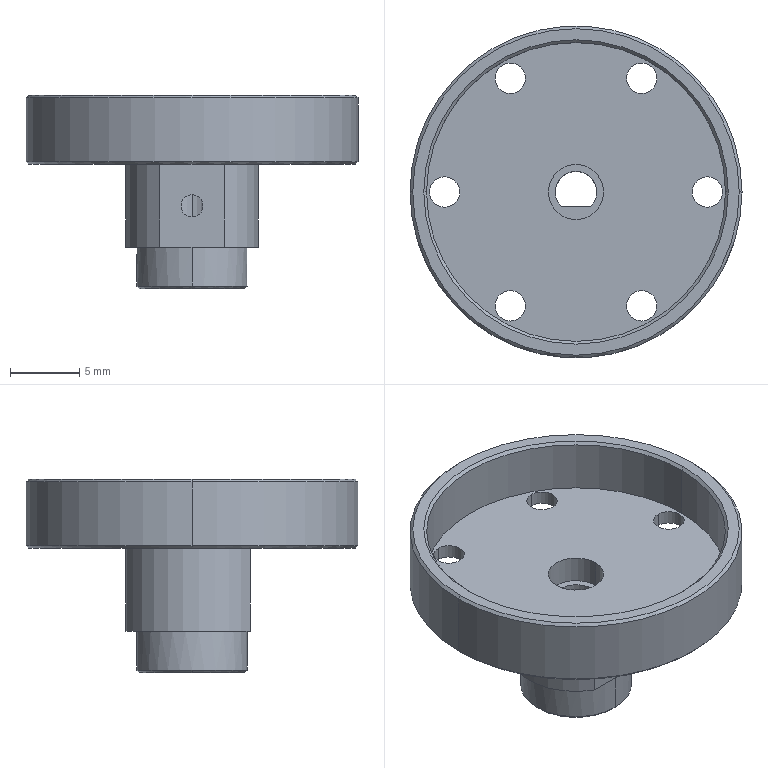NC program | NX | posted with a generic post | part box 24 x 24 x 14 mm
Whole program:
N10 G17 G21 G94 G90
(FLOOR_WALL , TOOL : D80)
N12 T19 M6
N14 G54
N16 G17 G0 G90 X-60. Y0. S6500 M3
N18 G43 Z30. H19
N20 Z3.
N22 G94 G1 Z0. F1500.
N24 X-57.
N26 X57.
N28 X60.
N30 Z3.
N32 G0 Z30.
N34 M5
(ADAPTIVE_MILLING , TOOL : D10)
N36 T15 M6
N38 G54
N40 G17 G0 G90 X-24.709 Y0.063 S9500 M3
N42 G43 Z30. H15
N44 Z-11.
N46 G94 G1 Z-14. F1000.
N48 X-23.929 Y-0.217 F3000.
N50 X-23.14 Y-0.473
N52 G3 X-22.062 Y0.063 R1.017
N54 X-21.301 Y3.126 R8.28
N56 X-21.019 Y12.993 R111.643
N58 G2 X-20.631 Y15.815 R6.542
N60 X-16.684 Y19.458 R7.316
N62 X-10.226 Y20.78 R19.548
N64 X2.021 Y20.985 R218.689
N66 X14.52 Y20.957 R545.112
N68 X18.704 Y18.063 R6.07
N70 X20.563 Y12.41 R13.683
N72 X20.97 Y3.05 R80.124
N74 G1 X20.978 Y1.55
N76 X20.983 Y-0.575
N78 X20.987 Y-3.825
N80 X20.988 Y-11.575
N82 Y-14.075
N84 X20.984 Y-14.2
N86 X20.977 Y-14.325
N88 X20.965 Y-14.45
N90 G2 X18.123 Y-18.666 R6.024
N92 X12.356 Y-20.57 R13.682
N94 X3.746 Y-20.965 R75.213
N96 G1 X2.621 Y-20.973
N98 X0.996 Y-20.98
N100 X-1.129 Y-20.984
N102 X-4.879 Y-20.987
N104 X-14.004 Y-20.988
N106 X-14.129 Y-20.986
N108 G2 X-18.331 Y-18.583 R5.703
N110 X-20.484 Y-12.917 R12.28
N112 X-20.964 Y-3.813 R67.206
N114 X-20.499 Y1.413 R49.975
N116 G3 X-20.03 Y11.524 R121.229
N118 G2 X-16.346 Y17.329 R7.752
N120 X-10.001 Y19.468 R15.489
N122 X-0.145 Y19.951 R80.815
N124 X11.604 Y19.947 R639.978
N126 X17.379 Y16.22 R7.712
N128 X19.482 Y9.861 R15.761
N130 X19.954 Y-0.247 R84.683
N132 X19.946 Y-11.621 R553.653
N134 X16.206 Y-17.388 R7.727
N136 X9.72 Y-19.498 R15.834
N138 X0.362 Y-19.949 R79.462
N140 X-11.637 Y-19.945 R478.691
N142 X-17.461 Y-16.084 R7.744
N144 X-19.515 Y-9.578 R16.213
N146 X-19.566 Y0.15 R42.335
N148 G3 X-19.067 Y9.385 R295.109
N150 G2 X-14.18 Y16.505 R9.108
N152 X-7.382 Y18.489 R18.641
N154 X3.103 Y18.942 R98.39
N156 X9.601 Y18.901 R98.045
N158 X16.439 Y14.21 R8.937
N160 X18.49 Y7.307 R18.265
N162 X18.94 Y-2.928 R95.698
N164 X18.906 Y-9.551 R109.181
N166 X14.255 Y-16.415 R8.913
N168 X7.233 Y-18.501 R18.411
N170 X-2.627 Y-18.937 R93.906
N172 X-9.5 Y-18.909 R118.757
N174 X-16.448 Y-14.185 R8.923
N176 X-18.535 Y-6.653 R18.416
N178 X-18.443 Y1.215 R58.227
N180 X-18.079 Y7.828 R136.173
N182 X-12.507 Y15.497 R10.026
N184 X-5.44 Y17.462 R20.584
N186 X7.418 Y17.888 R103.688
N188 X15.323 Y12.702 R9.73
N190 X17.406 Y5.803 R19.282
N192 X17.917 Y-4.303 R87.187
N194 X17.696 Y-8.788 R21.352
N196 X12.475 Y-15.447 R9.836
N198 X5.299 Y-17.472 R20.106
N200 X-7.435 Y-17.885 R103.812
N202 X-15.329 Y-12.682 R9.719
N204 X-17.376 Y-4.891 R18.076
N206 X-17.104 Y6.222 R84.007
N208 X-10.954 Y14.491 R10.754
N210 X-5.591 Y16.165 R19.739
N212 G1 X-4.308 Y16.597
N214 X-4.233 Y16.617
N216 X-1.841 Y17.048
N218 X-1.764 Y17.056
N220 G2 X3.23 Y17.012 R41.186
N222 X8.297 Y16.393 R17.013
N224 X14.624 Y10.53 R10.801
N226 X16.111 Y5.758 R19.717
N228 G1 X16.487 Y4.713
N230 X16.507 Y4.643
N232 G2 X17.149 Y0.012 R19.905
N234 G3 X16.904 Y-5.606 R192.191
N236 G2 X11.08 Y-14.346 R10.491
N238 X5.747 Y-16.114 R18.666
N240 G1 X4.848 Y-16.448
N242 X4.776 Y-16.469
N244 G2 X-0.019 Y-17.149 R19.964
N246 G3 X-5.637 Y-16.902 R229.027
N248 G2 X-14.514 Y-10.707 R10.491
N250 X-15.859 Y-6.426 R17.286
N252 G1 X-16.437 Y-4.886
N254 X-16.458 Y-4.812
N256 G2 X-17.148 Y0.051 R19.974
N258 G1 X-16.965 Y2.493
N260 X-16.954 Y2.57
N262 G2 X-15.648 Y7.316 R27.58
N264 X-13.008 Y11.136 R11.482
N266 X-10.896 Y13.241 R19.934
N268 G1 X-8.914 Y14.648
N270 X-8.848 Y14.688
N272 X-6.683 Y15.791
N274 X-6.611 Y15.821
N276 X-5.545 Y16.181
N278 X-4.233 Y16.617
N280 X-1.764 Y17.056
N282 X0.734 Y17.132
N284 X3.156 Y16.854
N286 X3.233 Y16.84
N288 G2 X8.077 Y15.188 R22.325
N290 X13.269 Y10.861 R19.685
N292 X15.717 Y6.857 R19.804
N294 G1 X16.139 Y5.681
N296 G3 X17.954 Y6.829 R-1.1
N298 G1 X6.864 Y17.977
N300 G3 X5.653 Y16.189 R-1.1
N302 G2 X9.829 Y14.051 R19.797
N304 G1 X10.413 Y13.581
N306 X11.659 Y12.574
N308 G2 X14.631 Y8.943 R20.021
N310 X16.507 Y4.643 R20.021
N312 X17.149 Y0.012 R20.111
N314 G1 X16.979 Y-2.397
N316 X16.968 Y-2.472
N318 G2 X15.096 Y-8.247 R20.663
N320 X13.544 Y-10.451 R12.904
N322 G1 X12.945 Y-11.245
N324 X12.896 Y-11.302
N326 G2 X9.206 Y-14.467 R19.857
N328 G1 X7.131 Y-15.594
N330 X7.062 Y-15.625
N332 X5.656 Y-16.148
N334 G3 X6.833 Y-17.941 R-1.1
N336 G1 X18.26 Y-6.034
N338 G3 X16.437 Y-4.886 R-1.1
N340 G2 X14.368 Y-9.36 R19.883
N342 G1 X13.539 Y-10.457
N344 X12.896 Y-11.302
N346 X11.164 Y-13.016
N348 X9.206 Y-14.467
N350 X7.062 Y-15.625
N352 X4.776 Y-16.469
N354 X2.393 Y-16.98
N356 X-0.019 Y-17.149
N358 X-2.393 Y-16.98
N360 X-2.468 Y-16.969
N362 G2 X-8.322 Y-15.053 R20.327
N364 X-10.38 Y-13.599 R12.851
N366 G1 X-11.164 Y-13.016
N368 X-11.221 Y-12.966
N370 G2 X-14.409 Y-9.296 R19.854
N372 G1 X-15.564 Y-7.198
N374 X-15.596 Y-7.128
N376 X-15.859 Y-6.426
N378 G3 X-17.631 Y-7.624 R-1.1
N380 G1 X-5.974 Y-18.29
N382 G3 X-4.848 Y-16.448 R-1.1
N384 G2 X-9.269 Y-14.426 R19.857
N386 G1 X-10.473 Y-13.53
N388 G3 X-11.229 Y-13.345 R1.027
N390 G1 X-11.962 Y-13.464
N392 X-13.937 Y-13.783 Z-13.9
N394 G2 X-14.973 Y-13.53 R1.086
N396 X-16.017 Y-12.377 R9.067
N398 G1 X-16.944 Y-10.932
N400 X-17.851 Y-9.475
N402 G2 X-19.849 Y-2.989 R15.613
N404 G1 X-20.317 Y2.69
N406 G2 X-19.529 Y3.751 R1.005
N408 G1 X-19.251 Y3.81
N410 X-17.295 Y4.226 Z-14.
N412 G3 X-16.42 Y4.94 R1.044
N414 G1 X-16.398 Y5.015
N416 X-15.524 Y7.282
N418 X-15.491 Y7.353
N420 X-14.296 Y9.469
N422 X-14.253 Y9.533
N424 X-12.949 Y11.211
N426 G3 X-12.926 Y12.419 R1.017
N428 G1 X-13.921 Y13.807
N430 Z-11.
N432 G0 Z30.
(ADAPTIVE_MILLING_COPY , TOOL : D10)
N434 X3.265 Y3.084
N436 Z3.
N438 G3 X3.265 Y3.084 Z2.506 I-3.272 J-3.089 F1000.
N440 X3.265 Y3.084 Z2.013 I-3.272 J-3.089
N442 X3.265 Y3.084 Z1.519 I-3.272 J-3.089
N444 X3.265 Y3.084 Z1.026 I-3.272 J-3.089
N446 X3.265 Y3.084 Z0.532 I-3.272 J-3.089
N448 X3.265 Y3.084 Z0.039 I-3.272 J-3.089
N450 X3.265 Y3.084 Z-0.455 I-3.272 J-3.089
N452 X3.265 Y3.084 Z-0.948 I-3.272 J-3.089
N454 X3.265 Y3.084 Z-1.442 I-3.272 J-3.089
N456 X3.265 Y3.084 Z-1.935 I-3.272 J-3.089
N458 X3.265 Y3.084 Z-2.429 I-3.272 J-3.089
N460 X3.265 Y3.084 Z-2.922 I-3.272 J-3.089
N462 X3.265 Y3.084 Z-3.416 I-3.272 J-3.089
N464 X4.493 Y-0.005 Z-3.85 R-4.5
N466 X3.671 Y-2.611 R-4.501 F3000.
N468 X-0.999 Y4.865 R4.671
N470 X3.576 Y-3.479 R-4.978
N472 X-1.657 Y5.205 R5.195
N474 X3.671 Y-4.091 R-5.477
N476 X5.235 Y-1.957 R5.961
N478 X5.632 Y0.167 R5.3
N480 X0.038 Y5.633 R5.695
N482 X-4.908 Y2.763 R5.788
N484 X-5.483 Y-1.313 R5.926
N486 X5.499 Y-1.168 R5.633
N488 X4.493 Y-0.032 R1.014
N490 G1 X3.116 Y-0.038
N492 Z-0.85
N494 G0 Z30.
N496 M5
(ZLEVEL_PROFILE_COPY_1_COPY_COPY_1 , TOOL : D10JING)
N498 T14 M6
N500 G54
N502 G17 G0 G90 X-18.925 Y-1.689 S9500 M3
N504 G43 Z30. H14
N506 Z-13.
N508 G94 G1 Z-14. F1000.
N510 X-17.5 Y-0.866
N512 G3 X-17. Y0. R1.
N514 G1 Y0.024 F1200.
N516 G2 X0.024 Y17. R17.
N518 X-17. Y0. R-17.
N520 G3 X-17.5 Y0.866 R1.
N522 G1 X-18.925 Y1.689
N524 Z-13.
N526 G0 Z30.
(FLOOR_WALL_1 , TOOL : D10JING)
N528 X0. Y-2.8
N530 Z-1.
N532 G1 Z-4. F1250.
N534 Y0.2
N536 G3 X-0.2 Y0. R0.2
N538 X0. Y0.2 R-0.2
N540 G1 Y5.2
N542 G3 X-5.2 Y0. R5.2
N544 X0. Y5.2 R-5.2
N546 G1 Y2.2
N548 Y5.7
N550 G3 X-5.7 Y0. R5.7
N552 X0. Y5.7 R-5.7
N554 G1 Y2.7
N556 Z-1.
N558 G0 Z30.
N560 M5
(HOLE_MILLING , TOOL : D3)
N562 T16 M6
N564 G54
N566 G17 G0 G90 X0. Y0. S9500 M3
N568 G43 Z30. H16
N570 Z-3.5
N572 G94 G3 X0.25 Y-0.25 R0.25 F1250.
N574 X0.5 Y0. R0.25
N576 X0.5 Y0. Z-3.7 I-0.5 J0.
N578 X0.5 Y0. Z-3.9 I-0.5 J0.
N580 X0.5 Y0. Z-4.1 I-0.5 J0.
N582 X0.5 Y0. Z-4.3 I-0.5 J0.
N584 X0.5 Y0. Z-4.5 I-0.5 J0.
N586 X0.5 Y0. Z-4.7 I-0.5 J0.
N588 X0.5 Y0. Z-4.9 I-0.5 J0.
N590 X0.5 Y0. Z-5.1 I-0.5 J0.
N592 X0.5 Y0. Z-5.3 I-0.5 J0.
N594 X0.5 Y0. Z-5.5 I-0.5 J0.
N596 X0.5 Y0. Z-5.7 I-0.5 J0.
N598 X0.5 Y0. Z-5.9 I-0.5 J0.
N600 X-0.5 Y0. Z-6. I-0.5 J0.
N602 X0. Y-0.5 R0.5
N604 X-0.5 Y0. R-0.5
N606 X-0.25 Y-0.25 R0.25
N608 X0. Y0. R0.25
N610 G0 Z30.
N612 M5
(PLANAR_MILL_COPY_COPY_COPY_COPY_COPY_COPY_1 , TOOL : D6A45)
N614 T01 M6
N616 G54
N618 G17 G0 G90 X-13.3 Y-0.866 S9500 M3
N620 G43 Z30. H1
N622 Z0.5
N624 G94 G1 Z-1. F1250.
N626 G3 X-12.8 Y0. R1.
N628 G2 X0. Y12.8 R12.8
N630 X-12.8 Y0. R-12.8
N632 G3 X-13.3 Y0.866 R1.
N634 G1 Z0.5
N636 G0 Z30.
N638 X9.5 Y-0.866
N640 Z0.5
N642 G1 Z-1.
N644 G3 X10. Y0. R1.
N646 X0. Y10. R10.
N648 X10. Y0. R-10.
N650 X9.5 Y0.866 R1.
N652 G1 Z0.5
N654 G0 Z30.
N656 M5
(刀补 , TOOL : D10JING)
N658 T14 M6
N660 G54
N662 G17 G0 G90 X2.75 Y0. S9500 M3
N664 G43 Z30. H14
N666 Z-1.
N668 G94 G1 Z-4. F1250.
N670 G41 X5.75 D14
N672 G3 X0. Y5.75 R5.75
N674 X5.75 Y0. R-5.75
N676 G40
N678 G1 X2.75
N680 Z-1.
N682 G0 Z30.
N684 M5
N686 M2